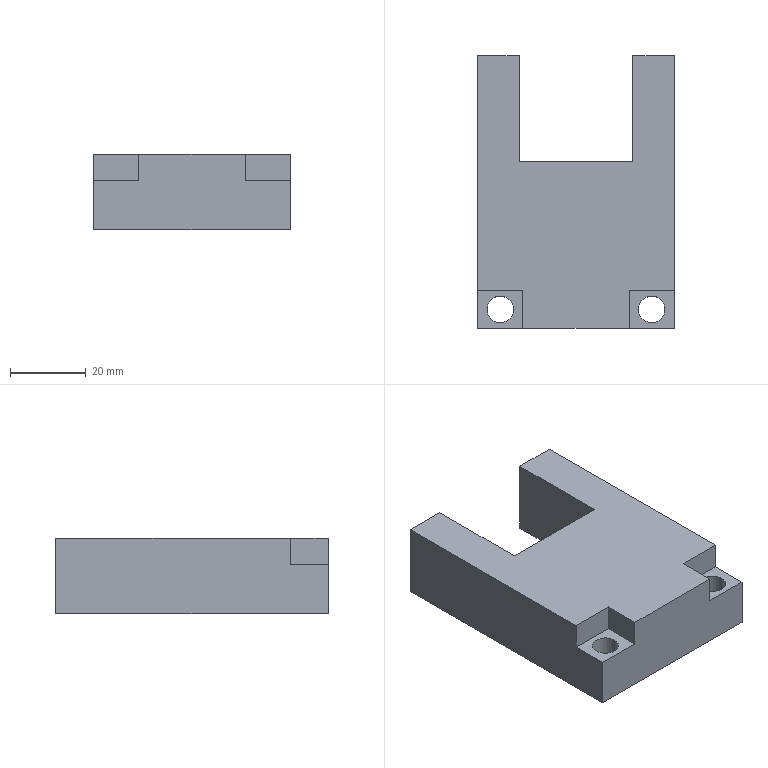Part | 1 solid | 20 faces | box 52 x 72 x 20 mm | volume 55399 mm3 | plane 16 | cylinder 4 | commonest cylinder face diameters 7 x4
STEP:
#1=CARTESIAN_POINT('',(23.5,-31.,0.));
#2=VERTEX_POINT('',#1);
#3=CARTESIAN_POINT('',(16.5,-31.,0.));
#4=VERTEX_POINT('',#3);
#5=CARTESIAN_POINT('',(20.,-31.,0.));
#6=DIRECTION('',(0.,0.,-1.));
#7=DIRECTION('',(-1.,0.,0.));
#8=AXIS2_PLACEMENT_3D('',#5,#6,#7);
#9=CIRCLE('',#8,3.5);
#10=EDGE_CURVE('',#2,#4,#9,.T.);
#11=ORIENTED_EDGE('',*,*,#10,.T.);
#12=CARTESIAN_POINT('',(16.5,-31.,13.));
#13=VERTEX_POINT('',#12);
#14=CARTESIAN_POINT('',(16.5,-31.,-32.));
#15=DIRECTION('',(0.,0.,1.));
#16=VECTOR('',#15,1000.);
#17=LINE('',#14,#16);
#18=EDGE_CURVE('',#4,#13,#17,.T.);
#19=ORIENTED_EDGE('',*,*,#18,.T.);
#20=CARTESIAN_POINT('',(23.5,-31.,13.));
#21=VERTEX_POINT('',#20);
#22=CARTESIAN_POINT('',(20.,-31.,13.));
#23=DIRECTION('',(0.,0.,1.));
#24=DIRECTION('',(1.,0.,0.));
#25=AXIS2_PLACEMENT_3D('',#22,#23,#24);
#26=CIRCLE('',#25,3.5);
#27=EDGE_CURVE('',#13,#21,#26,.T.);
#28=ORIENTED_EDGE('',*,*,#27,.T.);
#29=CARTESIAN_POINT('',(23.5,-31.,-32.));
#30=DIRECTION('',(0.,0.,1.));
#31=VECTOR('',#30,1000.);
#32=LINE('',#29,#31);
#33=EDGE_CURVE('',#2,#21,#32,.T.);
#34=ORIENTED_EDGE('',*,*,#33,.F.);
#35=EDGE_LOOP('',(#11,#19,#28,#34));
#36=FACE_OUTER_BOUND('',#35,.T.);
#37=CARTESIAN_POINT('',(20.,-31.,-32.));
#38=DIRECTION('',(0.,0.,1.));
#39=DIRECTION('',(1.,0.,0.));
#40=AXIS2_PLACEMENT_3D('',#37,#38,#39);
#41=CYLINDRICAL_SURFACE('',#40,3.5);
#42=ADVANCED_FACE('',(#36),#41,.F.);
#43=CARTESIAN_POINT('',(-16.5,-31.,0.));
#44=VERTEX_POINT('',#43);
#45=CARTESIAN_POINT('',(-23.5,-31.,0.));
#46=VERTEX_POINT('',#45);
#47=CARTESIAN_POINT('',(-20.,-31.,0.));
#48=DIRECTION('',(0.,0.,-1.));
#49=DIRECTION('',(-1.,0.,0.));
#50=AXIS2_PLACEMENT_3D('',#47,#48,#49);
#51=CIRCLE('',#50,3.5);
#52=EDGE_CURVE('',#44,#46,#51,.T.);
#53=ORIENTED_EDGE('',*,*,#52,.T.);
#54=CARTESIAN_POINT('',(-23.5,-31.,13.));
#55=VERTEX_POINT('',#54);
#56=CARTESIAN_POINT('',(-23.5,-31.,-32.));
#57=DIRECTION('',(0.,0.,1.));
#58=VECTOR('',#57,1000.);
#59=LINE('',#56,#58);
#60=EDGE_CURVE('',#46,#55,#59,.T.);
#61=ORIENTED_EDGE('',*,*,#60,.T.);
#62=CARTESIAN_POINT('',(-16.5,-31.,13.));
#63=VERTEX_POINT('',#62);
#64=CARTESIAN_POINT('',(-20.,-31.,13.));
#65=DIRECTION('',(0.,0.,-1.));
#66=DIRECTION('',(-1.,0.,0.));
#67=AXIS2_PLACEMENT_3D('',#64,#65,#66);
#68=CIRCLE('',#67,3.5);
#69=EDGE_CURVE('',#63,#55,#68,.T.);
#70=ORIENTED_EDGE('',*,*,#69,.F.);
#71=CARTESIAN_POINT('',(-16.5,-31.,-32.));
#72=DIRECTION('',(0.,0.,1.));
#73=VECTOR('',#72,1000.);
#74=LINE('',#71,#73);
#75=EDGE_CURVE('',#44,#63,#74,.T.);
#76=ORIENTED_EDGE('',*,*,#75,.F.);
#77=EDGE_LOOP('',(#53,#61,#70,#76));
#78=FACE_OUTER_BOUND('',#77,.T.);
#79=CARTESIAN_POINT('',(-20.,-31.,-32.));
#80=DIRECTION('',(0.,0.,1.));
#81=DIRECTION('',(1.,0.,0.));
#82=AXIS2_PLACEMENT_3D('',#79,#80,#81);
#83=CYLINDRICAL_SURFACE('',#82,3.5);
#84=ADVANCED_FACE('',(#78),#83,.F.);
#85=CARTESIAN_POINT('',(-15.,36.,20.));
#86=VERTEX_POINT('',#85);
#87=CARTESIAN_POINT('',(-26.,36.,20.));
#88=VERTEX_POINT('',#87);
#89=CARTESIAN_POINT('',(-26.,36.,20.));
#90=DIRECTION('',(-1.,0.,0.));
#91=VECTOR('',#90,1000.);
#92=LINE('',#89,#91);
#93=EDGE_CURVE('',#86,#88,#92,.T.);
#94=ORIENTED_EDGE('',*,*,#93,.F.);
#95=CARTESIAN_POINT('',(-15.,36.,0.));
#96=VERTEX_POINT('',#95);
#97=CARTESIAN_POINT('',(-15.,36.,0.));
#98=DIRECTION('',(0.,0.,1.));
#99=VECTOR('',#98,1000.);
#100=LINE('',#97,#99);
#101=EDGE_CURVE('',#96,#86,#100,.T.);
#102=ORIENTED_EDGE('',*,*,#101,.F.);
#103=CARTESIAN_POINT('',(-26.,36.,0.));
#104=VERTEX_POINT('',#103);
#105=CARTESIAN_POINT('',(-26.,36.,0.));
#106=DIRECTION('',(-1.,0.,0.));
#107=VECTOR('',#106,1000.);
#108=LINE('',#105,#107);
#109=EDGE_CURVE('',#96,#104,#108,.T.);
#110=ORIENTED_EDGE('',*,*,#109,.T.);
#111=CARTESIAN_POINT('',(-26.,36.,20.));
#112=DIRECTION('',(0.,0.,-1.));
#113=VECTOR('',#112,1000.);
#114=LINE('',#111,#113);
#115=EDGE_CURVE('',#88,#104,#114,.T.);
#116=ORIENTED_EDGE('',*,*,#115,.F.);
#117=EDGE_LOOP('',(#94,#102,#110,#116));
#118=FACE_OUTER_BOUND('',#117,.T.);
#119=CARTESIAN_POINT('',(-26.,36.,20.));
#120=DIRECTION('',(0.,-1.,0.));
#121=DIRECTION('',(0.,0.,-1.));
#122=AXIS2_PLACEMENT_3D('',#119,#120,#121);
#123=PLANE('',#122);
#124=ADVANCED_FACE('',(#118),#123,.F.);
#125=CARTESIAN_POINT('',(26.,-26.,20.));
#126=VERTEX_POINT('',#125);
#127=CARTESIAN_POINT('',(26.,36.,20.));
#128=VERTEX_POINT('',#127);
#129=CARTESIAN_POINT('',(26.,-36.,20.));
#130=DIRECTION('',(0.,1.,0.));
#131=VECTOR('',#130,1000.);
#132=LINE('',#129,#131);
#133=EDGE_CURVE('',#126,#128,#132,.T.);
#134=ORIENTED_EDGE('',*,*,#133,.F.);
#135=CARTESIAN_POINT('',(26.,-26.,13.));
#136=VERTEX_POINT('',#135);
#137=CARTESIAN_POINT('',(26.,-26.,13.));
#138=DIRECTION('',(0.,0.,1.));
#139=VECTOR('',#138,1000.);
#140=LINE('',#137,#139);
#141=EDGE_CURVE('',#136,#126,#140,.T.);
#142=ORIENTED_EDGE('',*,*,#141,.F.);
#143=CARTESIAN_POINT('',(26.,-36.,13.));
#144=VERTEX_POINT('',#143);
#145=CARTESIAN_POINT('',(26.,-36.,13.));
#146=DIRECTION('',(0.,1.,0.));
#147=VECTOR('',#146,1000.);
#148=LINE('',#145,#147);
#149=EDGE_CURVE('',#144,#136,#148,.T.);
#150=ORIENTED_EDGE('',*,*,#149,.F.);
#151=CARTESIAN_POINT('',(26.,-36.,0.));
#152=VERTEX_POINT('',#151);
#153=CARTESIAN_POINT('',(26.,-36.,20.));
#154=DIRECTION('',(0.,0.,-1.));
#155=VECTOR('',#154,1000.);
#156=LINE('',#153,#155);
#157=EDGE_CURVE('',#144,#152,#156,.T.);
#158=ORIENTED_EDGE('',*,*,#157,.T.);
#159=CARTESIAN_POINT('',(26.,36.,0.));
#160=VERTEX_POINT('',#159);
#161=CARTESIAN_POINT('',(26.,-36.,0.));
#162=DIRECTION('',(0.,1.,0.));
#163=VECTOR('',#162,1000.);
#164=LINE('',#161,#163);
#165=EDGE_CURVE('',#152,#160,#164,.T.);
#166=ORIENTED_EDGE('',*,*,#165,.T.);
#167=CARTESIAN_POINT('',(26.,36.,20.));
#168=DIRECTION('',(0.,0.,-1.));
#169=VECTOR('',#168,1000.);
#170=LINE('',#167,#169);
#171=EDGE_CURVE('',#128,#160,#170,.T.);
#172=ORIENTED_EDGE('',*,*,#171,.F.);
#173=EDGE_LOOP('',(#134,#142,#150,#158,#166,#172));
#174=FACE_OUTER_BOUND('',#173,.T.);
#175=CARTESIAN_POINT('',(26.,-36.,20.));
#176=DIRECTION('',(-1.,0.,0.));
#177=DIRECTION('',(0.,0.,1.));
#178=AXIS2_PLACEMENT_3D('',#175,#176,#177);
#179=PLANE('',#178);
#180=ADVANCED_FACE('',(#174),#179,.F.);
#181=CARTESIAN_POINT('',(15.,36.,0.));
#182=VERTEX_POINT('',#181);
#183=CARTESIAN_POINT('',(-26.,36.,0.));
#184=DIRECTION('',(-1.,0.,0.));
#185=VECTOR('',#184,1000.);
#186=LINE('',#183,#185);
#187=EDGE_CURVE('',#160,#182,#186,.T.);
#188=ORIENTED_EDGE('',*,*,#187,.T.);
#189=CARTESIAN_POINT('',(15.,36.,20.));
#190=VERTEX_POINT('',#189);
#191=CARTESIAN_POINT('',(15.,36.,0.));
#192=DIRECTION('',(0.,0.,1.));
#193=VECTOR('',#192,1000.);
#194=LINE('',#191,#193);
#195=EDGE_CURVE('',#182,#190,#194,.T.);
#196=ORIENTED_EDGE('',*,*,#195,.T.);
#197=CARTESIAN_POINT('',(-26.,36.,20.));
#198=DIRECTION('',(-1.,0.,0.));
#199=VECTOR('',#198,1000.);
#200=LINE('',#197,#199);
#201=EDGE_CURVE('',#128,#190,#200,.T.);
#202=ORIENTED_EDGE('',*,*,#201,.F.);
#203=ORIENTED_EDGE('',*,*,#171,.T.);
#204=EDGE_LOOP('',(#188,#196,#202,#203));
#205=FACE_OUTER_BOUND('',#204,.T.);
#206=CARTESIAN_POINT('',(-26.,36.,20.));
#207=DIRECTION('',(0.,-1.,0.));
#208=DIRECTION('',(0.,0.,-1.));
#209=AXIS2_PLACEMENT_3D('',#206,#207,#208);
#210=PLANE('',#209);
#211=ADVANCED_FACE('',(#205),#210,.F.);
#212=CARTESIAN_POINT('',(-26.,-26.,13.));
#213=VERTEX_POINT('',#212);
#214=CARTESIAN_POINT('',(-26.,-36.,13.));
#215=VERTEX_POINT('',#214);
#216=CARTESIAN_POINT('',(-26.,-36.,13.));
#217=DIRECTION('',(0.,-1.,0.));
#218=VECTOR('',#217,1000.);
#219=LINE('',#216,#218);
#220=EDGE_CURVE('',#213,#215,#219,.T.);
#221=ORIENTED_EDGE('',*,*,#220,.F.);
#222=CARTESIAN_POINT('',(-26.,-26.,20.));
#223=VERTEX_POINT('',#222);
#224=CARTESIAN_POINT('',(-26.,-26.,13.));
#225=DIRECTION('',(0.,0.,1.));
#226=VECTOR('',#225,1000.);
#227=LINE('',#224,#226);
#228=EDGE_CURVE('',#213,#223,#227,.T.);
#229=ORIENTED_EDGE('',*,*,#228,.T.);
#230=CARTESIAN_POINT('',(-26.,-36.,20.));
#231=DIRECTION('',(0.,-1.,0.));
#232=VECTOR('',#231,1000.);
#233=LINE('',#230,#232);
#234=EDGE_CURVE('',#88,#223,#233,.T.);
#235=ORIENTED_EDGE('',*,*,#234,.F.);
#236=ORIENTED_EDGE('',*,*,#115,.T.);
#237=CARTESIAN_POINT('',(-26.,-36.,0.));
#238=VERTEX_POINT('',#237);
#239=CARTESIAN_POINT('',(-26.,-36.,0.));
#240=DIRECTION('',(0.,-1.,0.));
#241=VECTOR('',#240,1000.);
#242=LINE('',#239,#241);
#243=EDGE_CURVE('',#104,#238,#242,.T.);
#244=ORIENTED_EDGE('',*,*,#243,.T.);
#245=CARTESIAN_POINT('',(-26.,-36.,20.));
#246=DIRECTION('',(0.,0.,-1.));
#247=VECTOR('',#246,1000.);
#248=LINE('',#245,#247);
#249=EDGE_CURVE('',#215,#238,#248,.T.);
#250=ORIENTED_EDGE('',*,*,#249,.F.);
#251=EDGE_LOOP('',(#221,#229,#235,#236,#244,#250));
#252=FACE_OUTER_BOUND('',#251,.T.);
#253=CARTESIAN_POINT('',(-26.,-36.,20.));
#254=DIRECTION('',(1.,0.,0.));
#255=DIRECTION('',(0.,0.,-1.));
#256=AXIS2_PLACEMENT_3D('',#253,#254,#255);
#257=PLANE('',#256);
#258=ADVANCED_FACE('',(#252),#257,.F.);
#259=CARTESIAN_POINT('',(14.,-36.,13.));
#260=VERTEX_POINT('',#259);
#261=CARTESIAN_POINT('',(26.,-36.,13.));
#262=DIRECTION('',(1.,0.,0.));
#263=VECTOR('',#262,1000.);
#264=LINE('',#261,#263);
#265=EDGE_CURVE('',#260,#144,#264,.T.);
#266=ORIENTED_EDGE('',*,*,#265,.F.);
#267=CARTESIAN_POINT('',(14.,-36.,20.));
#268=VERTEX_POINT('',#267);
#269=CARTESIAN_POINT('',(14.,-36.,13.));
#270=DIRECTION('',(0.,0.,1.));
#271=VECTOR('',#270,1000.);
#272=LINE('',#269,#271);
#273=EDGE_CURVE('',#260,#268,#272,.T.);
#274=ORIENTED_EDGE('',*,*,#273,.T.);
#275=CARTESIAN_POINT('',(-14.,-36.,20.));
#276=VERTEX_POINT('',#275);
#277=CARTESIAN_POINT('',(-26.,-36.,20.));
#278=DIRECTION('',(1.,0.,0.));
#279=VECTOR('',#278,1000.);
#280=LINE('',#277,#279);
#281=EDGE_CURVE('',#276,#268,#280,.T.);
#282=ORIENTED_EDGE('',*,*,#281,.F.);
#283=CARTESIAN_POINT('',(-14.,-36.,13.));
#284=VERTEX_POINT('',#283);
#285=CARTESIAN_POINT('',(-14.,-36.,13.));
#286=DIRECTION('',(0.,0.,1.));
#287=VECTOR('',#286,1000.);
#288=LINE('',#285,#287);
#289=EDGE_CURVE('',#284,#276,#288,.T.);
#290=ORIENTED_EDGE('',*,*,#289,.F.);
#291=CARTESIAN_POINT('',(-26.,-36.,13.));
#292=DIRECTION('',(1.,0.,0.));
#293=VECTOR('',#292,1000.);
#294=LINE('',#291,#293);
#295=EDGE_CURVE('',#215,#284,#294,.T.);
#296=ORIENTED_EDGE('',*,*,#295,.F.);
#297=ORIENTED_EDGE('',*,*,#249,.T.);
#298=CARTESIAN_POINT('',(-26.,-36.,0.));
#299=DIRECTION('',(1.,0.,0.));
#300=VECTOR('',#299,1000.);
#301=LINE('',#298,#300);
#302=EDGE_CURVE('',#238,#152,#301,.T.);
#303=ORIENTED_EDGE('',*,*,#302,.T.);
#304=ORIENTED_EDGE('',*,*,#157,.F.);
#305=EDGE_LOOP('',(#266,#274,#282,#290,#296,#297,#303,#304));
#306=FACE_OUTER_BOUND('',#305,.T.);
#307=CARTESIAN_POINT('',(-26.,-36.,20.));
#308=DIRECTION('',(0.,1.,0.));
#309=DIRECTION('',(0.,0.,1.));
#310=AXIS2_PLACEMENT_3D('',#307,#308,#309);
#311=PLANE('',#310);
#312=ADVANCED_FACE('',(#306),#311,.F.);
#313=ORIENTED_EDGE('',*,*,#281,.T.);
#314=CARTESIAN_POINT('',(14.,-26.,20.));
#315=VERTEX_POINT('',#314);
#316=CARTESIAN_POINT('',(14.,-36.,20.));
#317=DIRECTION('',(0.,-1.,0.));
#318=VECTOR('',#317,1000.);
#319=LINE('',#316,#318);
#320=EDGE_CURVE('',#315,#268,#319,.T.);
#321=ORIENTED_EDGE('',*,*,#320,.F.);
#322=CARTESIAN_POINT('',(26.,-26.,20.));
#323=DIRECTION('',(-1.,0.,0.));
#324=VECTOR('',#323,1000.);
#325=LINE('',#322,#324);
#326=EDGE_CURVE('',#126,#315,#325,.T.);
#327=ORIENTED_EDGE('',*,*,#326,.F.);
#328=ORIENTED_EDGE('',*,*,#133,.T.);
#329=ORIENTED_EDGE('',*,*,#201,.T.);
#330=CARTESIAN_POINT('',(15.,8.,20.));
#331=VERTEX_POINT('',#330);
#332=CARTESIAN_POINT('',(15.,36.,20.));
#333=DIRECTION('',(0.,1.,0.));
#334=VECTOR('',#333,1000.);
#335=LINE('',#332,#334);
#336=EDGE_CURVE('',#331,#190,#335,.T.);
#337=ORIENTED_EDGE('',*,*,#336,.F.);
#338=CARTESIAN_POINT('',(-15.,8.,20.));
#339=VERTEX_POINT('',#338);
#340=CARTESIAN_POINT('',(-15.,8.,20.));
#341=DIRECTION('',(1.,0.,0.));
#342=VECTOR('',#341,1000.);
#343=LINE('',#340,#342);
#344=EDGE_CURVE('',#339,#331,#343,.T.);
#345=ORIENTED_EDGE('',*,*,#344,.F.);
#346=CARTESIAN_POINT('',(-15.,36.,20.));
#347=DIRECTION('',(0.,-1.,0.));
#348=VECTOR('',#347,1000.);
#349=LINE('',#346,#348);
#350=EDGE_CURVE('',#86,#339,#349,.T.);
#351=ORIENTED_EDGE('',*,*,#350,.F.);
#352=ORIENTED_EDGE('',*,*,#93,.T.);
#353=ORIENTED_EDGE('',*,*,#234,.T.);
#354=CARTESIAN_POINT('',(-14.,-26.,20.));
#355=VERTEX_POINT('',#354);
#356=CARTESIAN_POINT('',(-26.,-26.,20.));
#357=DIRECTION('',(-1.,0.,0.));
#358=VECTOR('',#357,1000.);
#359=LINE('',#356,#358);
#360=EDGE_CURVE('',#355,#223,#359,.T.);
#361=ORIENTED_EDGE('',*,*,#360,.F.);
#362=CARTESIAN_POINT('',(-14.,-36.,20.));
#363=DIRECTION('',(0.,1.,0.));
#364=VECTOR('',#363,1000.);
#365=LINE('',#362,#364);
#366=EDGE_CURVE('',#276,#355,#365,.T.);
#367=ORIENTED_EDGE('',*,*,#366,.F.);
#368=EDGE_LOOP('',(#313,#321,#327,#328,#329,#337,#345,#351,#352,#353,#361,#367));
#369=FACE_OUTER_BOUND('',#368,.T.);
#370=CARTESIAN_POINT('',(0.,0.,20.));
#371=DIRECTION('',(0.,0.,-1.));
#372=DIRECTION('',(-1.,0.,0.));
#373=AXIS2_PLACEMENT_3D('',#370,#371,#372);
#374=PLANE('',#373);
#375=ADVANCED_FACE('',(#369),#374,.F.);
#376=ORIENTED_EDGE('',*,*,#10,.F.);
#377=CARTESIAN_POINT('',(20.,-31.,0.));
#378=DIRECTION('',(0.,0.,-1.));
#379=DIRECTION('',(-1.,0.,0.));
#380=AXIS2_PLACEMENT_3D('',#377,#378,#379);
#381=CIRCLE('',#380,3.5);
#382=EDGE_CURVE('',#4,#2,#381,.T.);
#383=ORIENTED_EDGE('',*,*,#382,.F.);
#384=EDGE_LOOP('',(#376,#383));
#385=FACE_BOUND('',#384,.T.);
#386=ORIENTED_EDGE('',*,*,#52,.F.);
#387=CARTESIAN_POINT('',(-20.,-31.,0.));
#388=DIRECTION('',(0.,0.,-1.));
#389=DIRECTION('',(-1.,0.,0.));
#390=AXIS2_PLACEMENT_3D('',#387,#388,#389);
#391=CIRCLE('',#390,3.5);
#392=EDGE_CURVE('',#46,#44,#391,.T.);
#393=ORIENTED_EDGE('',*,*,#392,.F.);
#394=EDGE_LOOP('',(#386,#393));
#395=FACE_BOUND('',#394,.T.);
#396=CARTESIAN_POINT('',(-15.,8.,0.));
#397=VERTEX_POINT('',#396);
#398=CARTESIAN_POINT('',(-15.,36.,0.));
#399=DIRECTION('',(0.,-1.,0.));
#400=VECTOR('',#399,1000.);
#401=LINE('',#398,#400);
#402=EDGE_CURVE('',#96,#397,#401,.T.);
#403=ORIENTED_EDGE('',*,*,#402,.T.);
#404=CARTESIAN_POINT('',(15.,8.,0.));
#405=VERTEX_POINT('',#404);
#406=CARTESIAN_POINT('',(-15.,8.,0.));
#407=DIRECTION('',(1.,0.,0.));
#408=VECTOR('',#407,1000.);
#409=LINE('',#406,#408);
#410=EDGE_CURVE('',#397,#405,#409,.T.);
#411=ORIENTED_EDGE('',*,*,#410,.T.);
#412=CARTESIAN_POINT('',(15.,36.,0.));
#413=DIRECTION('',(0.,1.,0.));
#414=VECTOR('',#413,1000.);
#415=LINE('',#412,#414);
#416=EDGE_CURVE('',#405,#182,#415,.T.);
#417=ORIENTED_EDGE('',*,*,#416,.T.);
#418=ORIENTED_EDGE('',*,*,#187,.F.);
#419=ORIENTED_EDGE('',*,*,#165,.F.);
#420=ORIENTED_EDGE('',*,*,#302,.F.);
#421=ORIENTED_EDGE('',*,*,#243,.F.);
#422=ORIENTED_EDGE('',*,*,#109,.F.);
#423=EDGE_LOOP('',(#403,#411,#417,#418,#419,#420,#421,#422));
#424=FACE_OUTER_BOUND('',#423,.T.);
#425=CARTESIAN_POINT('',(0.,0.,0.));
#426=DIRECTION('',(0.,0.,-1.));
#427=DIRECTION('',(-1.,0.,0.));
#428=AXIS2_PLACEMENT_3D('',#425,#426,#427);
#429=PLANE('',#428);
#430=ADVANCED_FACE('',(#385,#395,#424),#429,.T.);
#431=ORIENTED_EDGE('',*,*,#350,.T.);
#432=CARTESIAN_POINT('',(-15.,8.,0.));
#433=DIRECTION('',(0.,0.,1.));
#434=VECTOR('',#433,1000.);
#435=LINE('',#432,#434);
#436=EDGE_CURVE('',#397,#339,#435,.T.);
#437=ORIENTED_EDGE('',*,*,#436,.F.);
#438=ORIENTED_EDGE('',*,*,#402,.F.);
#439=ORIENTED_EDGE('',*,*,#101,.T.);
#440=EDGE_LOOP('',(#431,#437,#438,#439));
#441=FACE_OUTER_BOUND('',#440,.T.);
#442=CARTESIAN_POINT('',(-15.,36.,0.));
#443=DIRECTION('',(-1.,0.,0.));
#444=DIRECTION('',(0.,-1.,0.));
#445=AXIS2_PLACEMENT_3D('',#442,#443,#444);
#446=PLANE('',#445);
#447=ADVANCED_FACE('',(#441),#446,.F.);
#448=ORIENTED_EDGE('',*,*,#336,.T.);
#449=ORIENTED_EDGE('',*,*,#195,.F.);
#450=ORIENTED_EDGE('',*,*,#416,.F.);
#451=CARTESIAN_POINT('',(15.,8.,0.));
#452=DIRECTION('',(0.,0.,1.));
#453=VECTOR('',#452,1000.);
#454=LINE('',#451,#453);
#455=EDGE_CURVE('',#405,#331,#454,.T.);
#456=ORIENTED_EDGE('',*,*,#455,.T.);
#457=EDGE_LOOP('',(#448,#449,#450,#456));
#458=FACE_OUTER_BOUND('',#457,.T.);
#459=CARTESIAN_POINT('',(15.,36.,0.));
#460=DIRECTION('',(1.,0.,0.));
#461=DIRECTION('',(0.,0.,-1.));
#462=AXIS2_PLACEMENT_3D('',#459,#460,#461);
#463=PLANE('',#462);
#464=ADVANCED_FACE('',(#458),#463,.F.);
#465=ORIENTED_EDGE('',*,*,#344,.T.);
#466=ORIENTED_EDGE('',*,*,#455,.F.);
#467=ORIENTED_EDGE('',*,*,#410,.F.);
#468=ORIENTED_EDGE('',*,*,#436,.T.);
#469=EDGE_LOOP('',(#465,#466,#467,#468));
#470=FACE_OUTER_BOUND('',#469,.T.);
#471=CARTESIAN_POINT('',(-15.,8.,0.));
#472=DIRECTION('',(0.,-1.,0.));
#473=DIRECTION('',(0.,0.,-1.));
#474=AXIS2_PLACEMENT_3D('',#471,#472,#473);
#475=PLANE('',#474);
#476=ADVANCED_FACE('',(#470),#475,.F.);
#477=ORIENTED_EDGE('',*,*,#360,.T.);
#478=ORIENTED_EDGE('',*,*,#228,.F.);
#479=CARTESIAN_POINT('',(-14.,-26.,13.));
#480=VERTEX_POINT('',#479);
#481=CARTESIAN_POINT('',(-26.,-26.,13.));
#482=DIRECTION('',(-1.,0.,0.));
#483=VECTOR('',#482,1000.);
#484=LINE('',#481,#483);
#485=EDGE_CURVE('',#480,#213,#484,.T.);
#486=ORIENTED_EDGE('',*,*,#485,.F.);
#487=CARTESIAN_POINT('',(-14.,-26.,13.));
#488=DIRECTION('',(0.,0.,1.));
#489=VECTOR('',#488,1000.);
#490=LINE('',#487,#489);
#491=EDGE_CURVE('',#480,#355,#490,.T.);
#492=ORIENTED_EDGE('',*,*,#491,.T.);
#493=EDGE_LOOP('',(#477,#478,#486,#492));
#494=FACE_OUTER_BOUND('',#493,.T.);
#495=CARTESIAN_POINT('',(-26.,-26.,13.));
#496=DIRECTION('',(0.,1.,0.));
#497=DIRECTION('',(0.,0.,1.));
#498=AXIS2_PLACEMENT_3D('',#495,#496,#497);
#499=PLANE('',#498);
#500=ADVANCED_FACE('',(#494),#499,.F.);
#501=ORIENTED_EDGE('',*,*,#366,.T.);
#502=ORIENTED_EDGE('',*,*,#491,.F.);
#503=CARTESIAN_POINT('',(-14.,-36.,13.));
#504=DIRECTION('',(0.,1.,0.));
#505=VECTOR('',#504,1000.);
#506=LINE('',#503,#505);
#507=EDGE_CURVE('',#284,#480,#506,.T.);
#508=ORIENTED_EDGE('',*,*,#507,.F.);
#509=ORIENTED_EDGE('',*,*,#289,.T.);
#510=EDGE_LOOP('',(#501,#502,#508,#509));
#511=FACE_OUTER_BOUND('',#510,.T.);
#512=CARTESIAN_POINT('',(-14.,-36.,13.));
#513=DIRECTION('',(1.,0.,0.));
#514=DIRECTION('',(0.,0.,-1.));
#515=AXIS2_PLACEMENT_3D('',#512,#513,#514);
#516=PLANE('',#515);
#517=ADVANCED_FACE('',(#511),#516,.F.);
#518=ORIENTED_EDGE('',*,*,#69,.T.);
#519=CARTESIAN_POINT('',(-20.,-31.,13.));
#520=DIRECTION('',(0.,0.,-1.));
#521=DIRECTION('',(-1.,0.,0.));
#522=AXIS2_PLACEMENT_3D('',#519,#520,#521);
#523=CIRCLE('',#522,3.5);
#524=EDGE_CURVE('',#55,#63,#523,.T.);
#525=ORIENTED_EDGE('',*,*,#524,.T.);
#526=EDGE_LOOP('',(#518,#525));
#527=FACE_BOUND('',#526,.T.);
#528=ORIENTED_EDGE('',*,*,#220,.T.);
#529=ORIENTED_EDGE('',*,*,#295,.T.);
#530=ORIENTED_EDGE('',*,*,#507,.T.);
#531=ORIENTED_EDGE('',*,*,#485,.T.);
#532=EDGE_LOOP('',(#528,#529,#530,#531));
#533=FACE_OUTER_BOUND('',#532,.T.);
#534=CARTESIAN_POINT('',(0.,0.,13.));
#535=DIRECTION('',(0.,0.,-1.));
#536=DIRECTION('',(-1.,0.,0.));
#537=AXIS2_PLACEMENT_3D('',#534,#535,#536);
#538=PLANE('',#537);
#539=ADVANCED_FACE('',(#527,#533),#538,.F.);
#540=ORIENTED_EDGE('',*,*,#320,.T.);
#541=ORIENTED_EDGE('',*,*,#273,.F.);
#542=CARTESIAN_POINT('',(14.,-26.,13.));
#543=VERTEX_POINT('',#542);
#544=CARTESIAN_POINT('',(14.,-36.,13.));
#545=DIRECTION('',(0.,-1.,0.));
#546=VECTOR('',#545,1000.);
#547=LINE('',#544,#546);
#548=EDGE_CURVE('',#543,#260,#547,.T.);
#549=ORIENTED_EDGE('',*,*,#548,.F.);
#550=CARTESIAN_POINT('',(14.,-26.,13.));
#551=DIRECTION('',(0.,0.,1.));
#552=VECTOR('',#551,1000.);
#553=LINE('',#550,#552);
#554=EDGE_CURVE('',#543,#315,#553,.T.);
#555=ORIENTED_EDGE('',*,*,#554,.T.);
#556=EDGE_LOOP('',(#540,#541,#549,#555));
#557=FACE_OUTER_BOUND('',#556,.T.);
#558=CARTESIAN_POINT('',(14.,-36.,13.));
#559=DIRECTION('',(-1.,0.,0.));
#560=DIRECTION('',(0.,0.,1.));
#561=AXIS2_PLACEMENT_3D('',#558,#559,#560);
#562=PLANE('',#561);
#563=ADVANCED_FACE('',(#557),#562,.F.);
#564=ORIENTED_EDGE('',*,*,#326,.T.);
#565=ORIENTED_EDGE('',*,*,#554,.F.);
#566=CARTESIAN_POINT('',(26.,-26.,13.));
#567=DIRECTION('',(-1.,0.,0.));
#568=VECTOR('',#567,1000.);
#569=LINE('',#566,#568);
#570=EDGE_CURVE('',#136,#543,#569,.T.);
#571=ORIENTED_EDGE('',*,*,#570,.F.);
#572=ORIENTED_EDGE('',*,*,#141,.T.);
#573=EDGE_LOOP('',(#564,#565,#571,#572));
#574=FACE_OUTER_BOUND('',#573,.T.);
#575=CARTESIAN_POINT('',(26.,-26.,13.));
#576=DIRECTION('',(0.,1.,0.));
#577=DIRECTION('',(0.,0.,1.));
#578=AXIS2_PLACEMENT_3D('',#575,#576,#577);
#579=PLANE('',#578);
#580=ADVANCED_FACE('',(#574),#579,.F.);
#581=CARTESIAN_POINT('',(20.,-31.,13.));
#582=DIRECTION('',(0.,0.,1.));
#583=DIRECTION('',(1.,0.,0.));
#584=AXIS2_PLACEMENT_3D('',#581,#582,#583);
#585=CIRCLE('',#584,3.5);
#586=EDGE_CURVE('',#21,#13,#585,.T.);
#587=ORIENTED_EDGE('',*,*,#586,.F.);
#588=ORIENTED_EDGE('',*,*,#27,.F.);
#589=EDGE_LOOP('',(#587,#588));
#590=FACE_BOUND('',#589,.T.);
#591=ORIENTED_EDGE('',*,*,#149,.T.);
#592=ORIENTED_EDGE('',*,*,#570,.T.);
#593=ORIENTED_EDGE('',*,*,#548,.T.);
#594=ORIENTED_EDGE('',*,*,#265,.T.);
#595=EDGE_LOOP('',(#591,#592,#593,#594));
#596=FACE_OUTER_BOUND('',#595,.T.);
#597=CARTESIAN_POINT('',(0.,0.,13.));
#598=DIRECTION('',(0.,0.,1.));
#599=DIRECTION('',(1.,0.,0.));
#600=AXIS2_PLACEMENT_3D('',#597,#598,#599);
#601=PLANE('',#600);
#602=ADVANCED_FACE('',(#590,#596),#601,.T.);
#603=ORIENTED_EDGE('',*,*,#60,.F.);
#604=ORIENTED_EDGE('',*,*,#392,.T.);
#605=ORIENTED_EDGE('',*,*,#75,.T.);
#606=ORIENTED_EDGE('',*,*,#524,.F.);
#607=EDGE_LOOP('',(#603,#604,#605,#606));
#608=FACE_OUTER_BOUND('',#607,.T.);
#609=CARTESIAN_POINT('',(-20.,-31.,-32.));
#610=DIRECTION('',(0.,0.,1.));
#611=DIRECTION('',(1.,0.,0.));
#612=AXIS2_PLACEMENT_3D('',#609,#610,#611);
#613=CYLINDRICAL_SURFACE('',#612,3.5);
#614=ADVANCED_FACE('',(#608),#613,.F.);
#615=ORIENTED_EDGE('',*,*,#18,.F.);
#616=ORIENTED_EDGE('',*,*,#382,.T.);
#617=ORIENTED_EDGE('',*,*,#33,.T.);
#618=ORIENTED_EDGE('',*,*,#586,.T.);
#619=EDGE_LOOP('',(#615,#616,#617,#618));
#620=FACE_OUTER_BOUND('',#619,.T.);
#621=CARTESIAN_POINT('',(20.,-31.,-32.));
#622=DIRECTION('',(0.,0.,1.));
#623=DIRECTION('',(1.,0.,0.));
#624=AXIS2_PLACEMENT_3D('',#621,#622,#623);
#625=CYLINDRICAL_SURFACE('',#624,3.5);
#626=ADVANCED_FACE('',(#620),#625,.F.);
#627=CLOSED_SHELL('',(#42,#84,#124,#180,#211,#258,#312,#375,#430,#447,#464,#476,#500,#517,#539,#563,#580,#602,#614,#626));
#628=MANIFOLD_SOLID_BREP('',#627);
#629=CARTESIAN_POINT('',(0.,0.,0.));
#630=DIRECTION('',(0.,0.,1.));
#631=DIRECTION('',(1.,0.,0.));
#632=AXIS2_PLACEMENT_3D('',#629,#630,#631);
#633=(LENGTH_UNIT()NAMED_UNIT(*)SI_UNIT(.MILLI.,.METRE.));
#634=UNCERTAINTY_MEASURE_WITH_UNIT(LENGTH_MEASURE(0.00001),#633,'','');
#635=(NAMED_UNIT(*)PLANE_ANGLE_UNIT()SI_UNIT($,.RADIAN.));
#636=(NAMED_UNIT(*)SI_UNIT($,.STERADIAN.)SOLID_ANGLE_UNIT());
#637=(GEOMETRIC_REPRESENTATION_CONTEXT(3)GLOBAL_UNCERTAINTY_ASSIGNED_CONTEXT((#634))GLOBAL_UNIT_ASSIGNED_CONTEXT((#633,#635,#636))REPRESENTATION_CONTEXT('',''));
#638=ADVANCED_BREP_SHAPE_REPRESENTATION('',(#628,#632),#637);